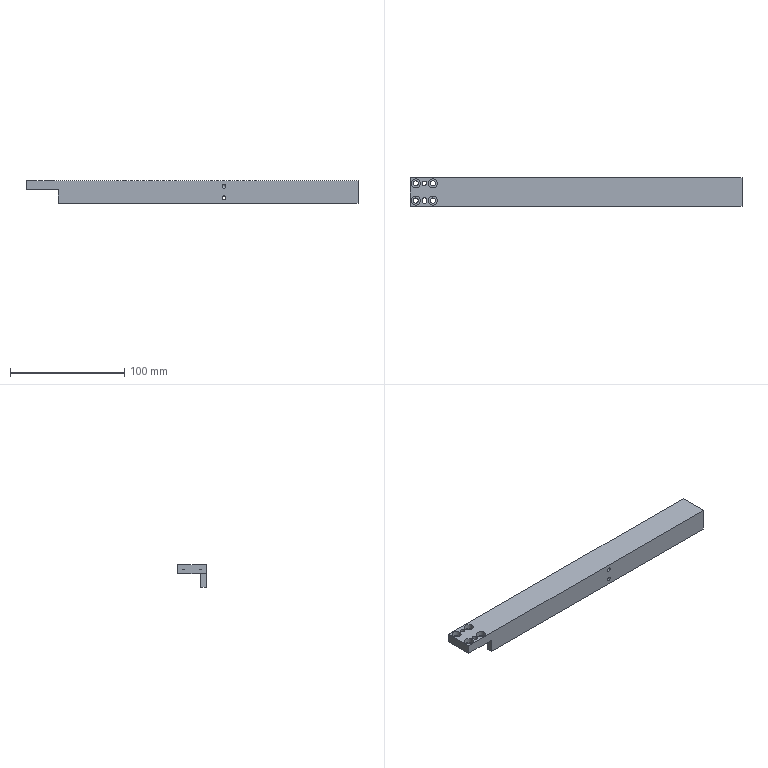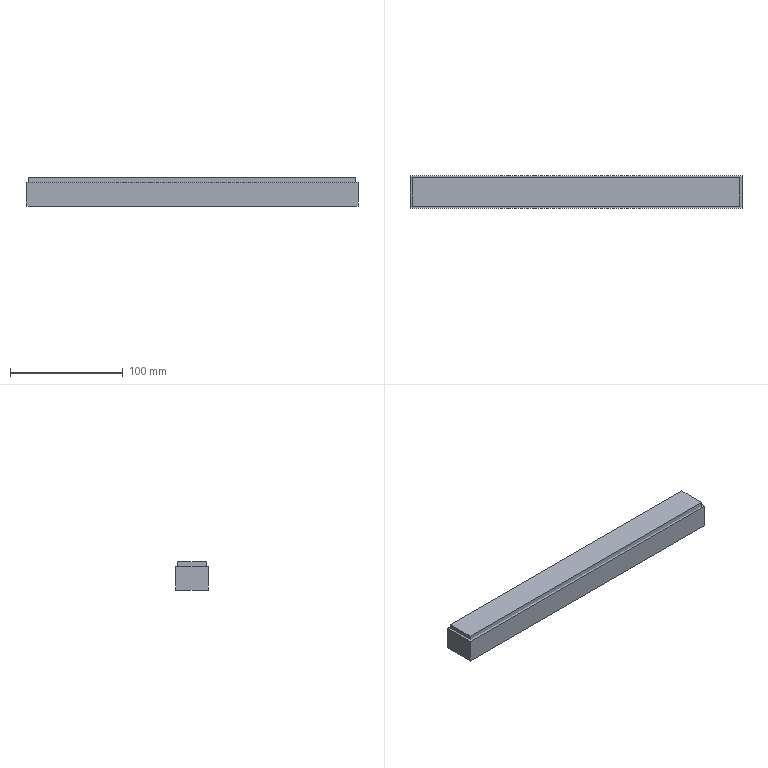CAM job | NX | 3-axis milling, drilling | part box 290 x 25 x 20 mm | stock box 294 x 29 x 25 mm
Tools:
number,name,description,diameter,corner_radius,flute_length,length,flutes
1,D50,Milling Tool-5 Parameters,50.0,0.0,50.0,75.0,2
2,D6A45,Milling Tool-5 Parameters,6.0,0.0,3.0,3.0,2
14,4.5ZT,Drilling Tool,4.5,0.0,35.0,50.0,2
12,2.5ZT,Drilling Tool,2.5,0.0,35.0,50.0,2
3,D10,Milling Tool-5 Parameters,10.0,0.0,50.0,75.0,2
4,D10JING,Milling Tool-5 Parameters,10.0,0.0,50.0,75.0,2
8,D6,Milling Tool-5 Parameters,6.0,0.0,50.0,75.0,2
20,D3,Milling Tool-5 Parameters,3.0,0.0,50.0,75.0,2
20,D6R0.5,Milling Tool-5 Parameters,6.0,0.5,50.0,75.0,2
Operations:
program,operation,operation_type,tool,method,geometry_group,spindle_rpm,surface_speed,feed_per_tooth,feed_cut,feed_plunge,cut_length_mm,path_length_mm,cut_time_min,machine_time_min
1-293-25-25毛胚-虎钳,FLOOR_WALL,VolumeBased25DMillingOperation,D50,METHOD,A,6500.0,1286.0,0.0962,1250.0,100.0,356.0,410.0,0.2848,0.2902
1-293-25-25毛胚-虎钳,DRILLING_COPY_1,Operation,D6A45,METHOD,A,3000.0,56.0,0.0333,200.0,0.0,27.6,177.839,0.138,0.153
1-293-25-25毛胚-虎钳,DRILLING_COPY_1_COPY_COPY_1_COPY_1_COPY,Operation,4.5ZT,METHOD,A,2000.0,18.0,0.03,120.0,0.0,55.408,225.707,0.4617,0.4788
1-293-25-25毛胚-虎钳,DRILLING_COPY_1_COPY_COPY_1_COPY_1_COPY_COPY,Operation,2.5ZT,METHOD,A,2000.0,18.0,0.03,120.0,0.0,26.502,130.811,0.2209,0.2313
1-293-25-25毛胚-虎钳,ZLEVEL_PROFILE,ZLevelMilling,D10,METHOD,A,7000.0,219.0,0.2143,3000.0,1000.0,13347.609,13424.609,4.481,4.489
1-293-25-25毛胚-虎钳,ZLEVEL_PROFILE_COPY_COPY_1_COPY_COPY_COPY_1,ZLevelMilling,D10JING,METHOD,A,7000.0,219.0,0.0714,1000.0,100.0,664.548,764.548,0.6645,0.6745
1-293-25-25毛胚-虎钳,HOLE_MILLING_1,CylinderMilling,D6,METHOD,A,7000.0,131.0,0.1071,1500.0,100.0,284.779,585.379,0.1899,0.2199
1-293-25-25毛胚-虎钳,ZLEVEL_PROFILE_COPY_1_COPY,ZLevelMilling,D3,METHOD,A,7000.0,65.0,0.0929,1300.0,1000.0,263.194,410.602,0.2139,0.2286
1-293-25-25毛胚-虎钳,ZLEVEL_PROFILE_COPY_1_COPY_COPY_COPY_COPY_2_COPY,ZLevelMilling,D6A45,METHOD,A,7000.0,131.0,0.0714,1000.0,1000.0,753.613,1538.126,0.7536,0.8321
1-293-25-25毛胚-虎钳,刀补10_COPY,ZLevelMilling,D3,METHOD,A,7000.0,87.0,0.0607,850.0,1000.0,73.319,223.961,0.0859,0.1009
2-293-25-25毛胚_虎钳,FLOOR_WALL_COPY,VolumeBased25DMillingOperation,D50,METHOD,B,6500.0,1286.0,0.0962,1250.0,100.0,1760.0,3394.001,1.408,1.571
2-293-25-25毛胚_虎钳,FLOOR_WALL_1,VolumeBased25DMillingOperation,D10,METHOD,B,7000.0,219.0,0.2143,3000.0,1000.0,6582.844,7475.951,2.215,2.304
2-293-25-25毛胚_虎钳,FLOOR_WALL_1_COPY_1,VolumeBased25DMillingOperation,D10JING,METHOD,B,7000.0,87.0,0.0714,1000.0,100.0,2194.421,2294.241,2.194,2.205
2-293-25-25毛胚_虎钳,ZLEVEL_PROFILE_COPY_COPY_1_COPY_COPY_COPY_1_1,ZLevelMilling,D10JING,METHOD,B,7000.0,219.0,0.0714,1000.0,100.0,277.828,361.828,0.2778,0.2862
2-293-25-25毛胚_虎钳,ZLEVEL_PROFILE_COPY_COPY_1_COPY_COPY_COPY_1_COPY_COPY,ZLevelMilling,D6R0.5,METHOD,B,7000.0,131.0,0.2143,3000.0,1000.0,1870.321,1957.536,0.6241,0.6328
2-293-25-25毛胚_虎钳,ZLEVEL_PROFILE_COPY_1_COPY_COPY_COPY_COPY_2_COPY_COPY,ZLevelMilling,D6A45,METHOD,B,7000.0,131.0,0.0714,1000.0,1000.0,540.646,602.646,0.5406,0.5468
2-293-25-25毛胚_虎钳,ZLEVEL_PROFILE_COPY_1_COPY_COPY_COPY_COPY_2_COPY_COPY_COPY,ZLevelMilling,D6A45,METHOD,B,7000.0,131.0,0.0714,1000.0,1000.0,401.622,1336.329,0.4016,0.4951
2-293-25-25毛胚_虎钳,刀补4,ZLevelMilling,D10JING,METHOD,B,7000.0,219.0,0.0714,1000.0,100.0,20.997,102.997,0.021,0.0292